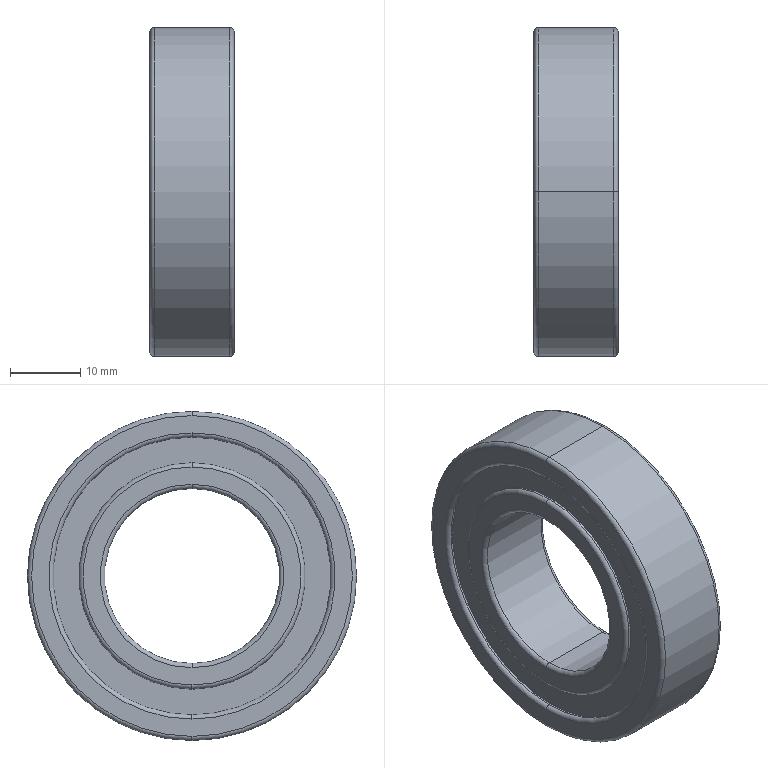Part | SolidWorks | features Revolution 5, CirPattern 2, RefAxis 1, RevCut 1 | 17 solids | 212 faces | box 12 x 47 x 47 mm | volume 11391 mm3 | cylinder 82 | sphere 68 | plane 40 | torus 22 | commonest cylinder face diameters 34.9 x31 37.1 x31 32.333 x8 39.667 x8 25 x2 47 x2